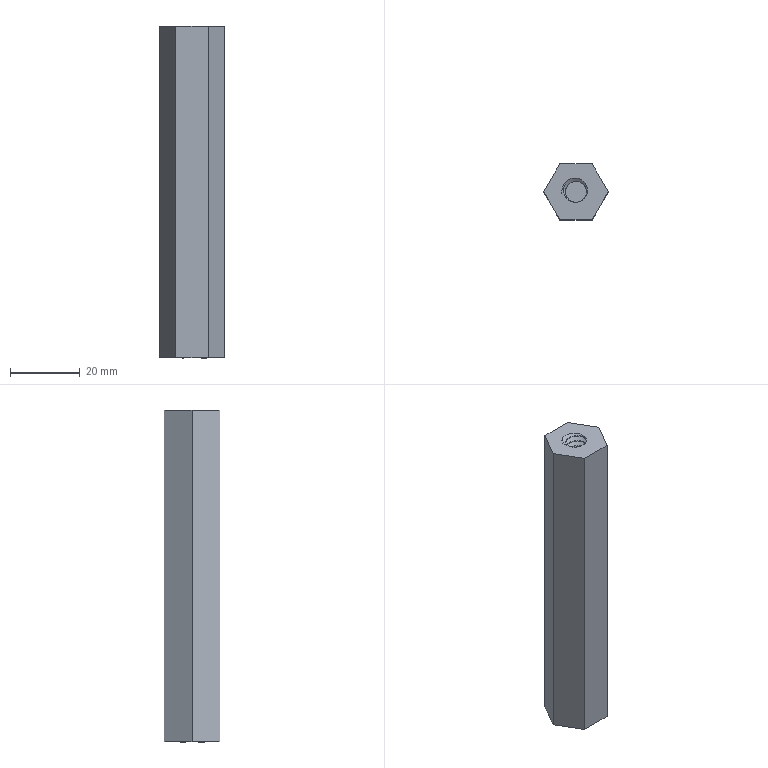Part | SolidWorks | features Helix 2, ICE 2, SweepCut 2, Extrusion 1 | 1 solid | 81 faces | box 18.475 x 16 x 95 mm | volume 19634 mm3 | cylinder 65 | plane 12 | spline 4 | commonest cylinder face diameters 6 x65